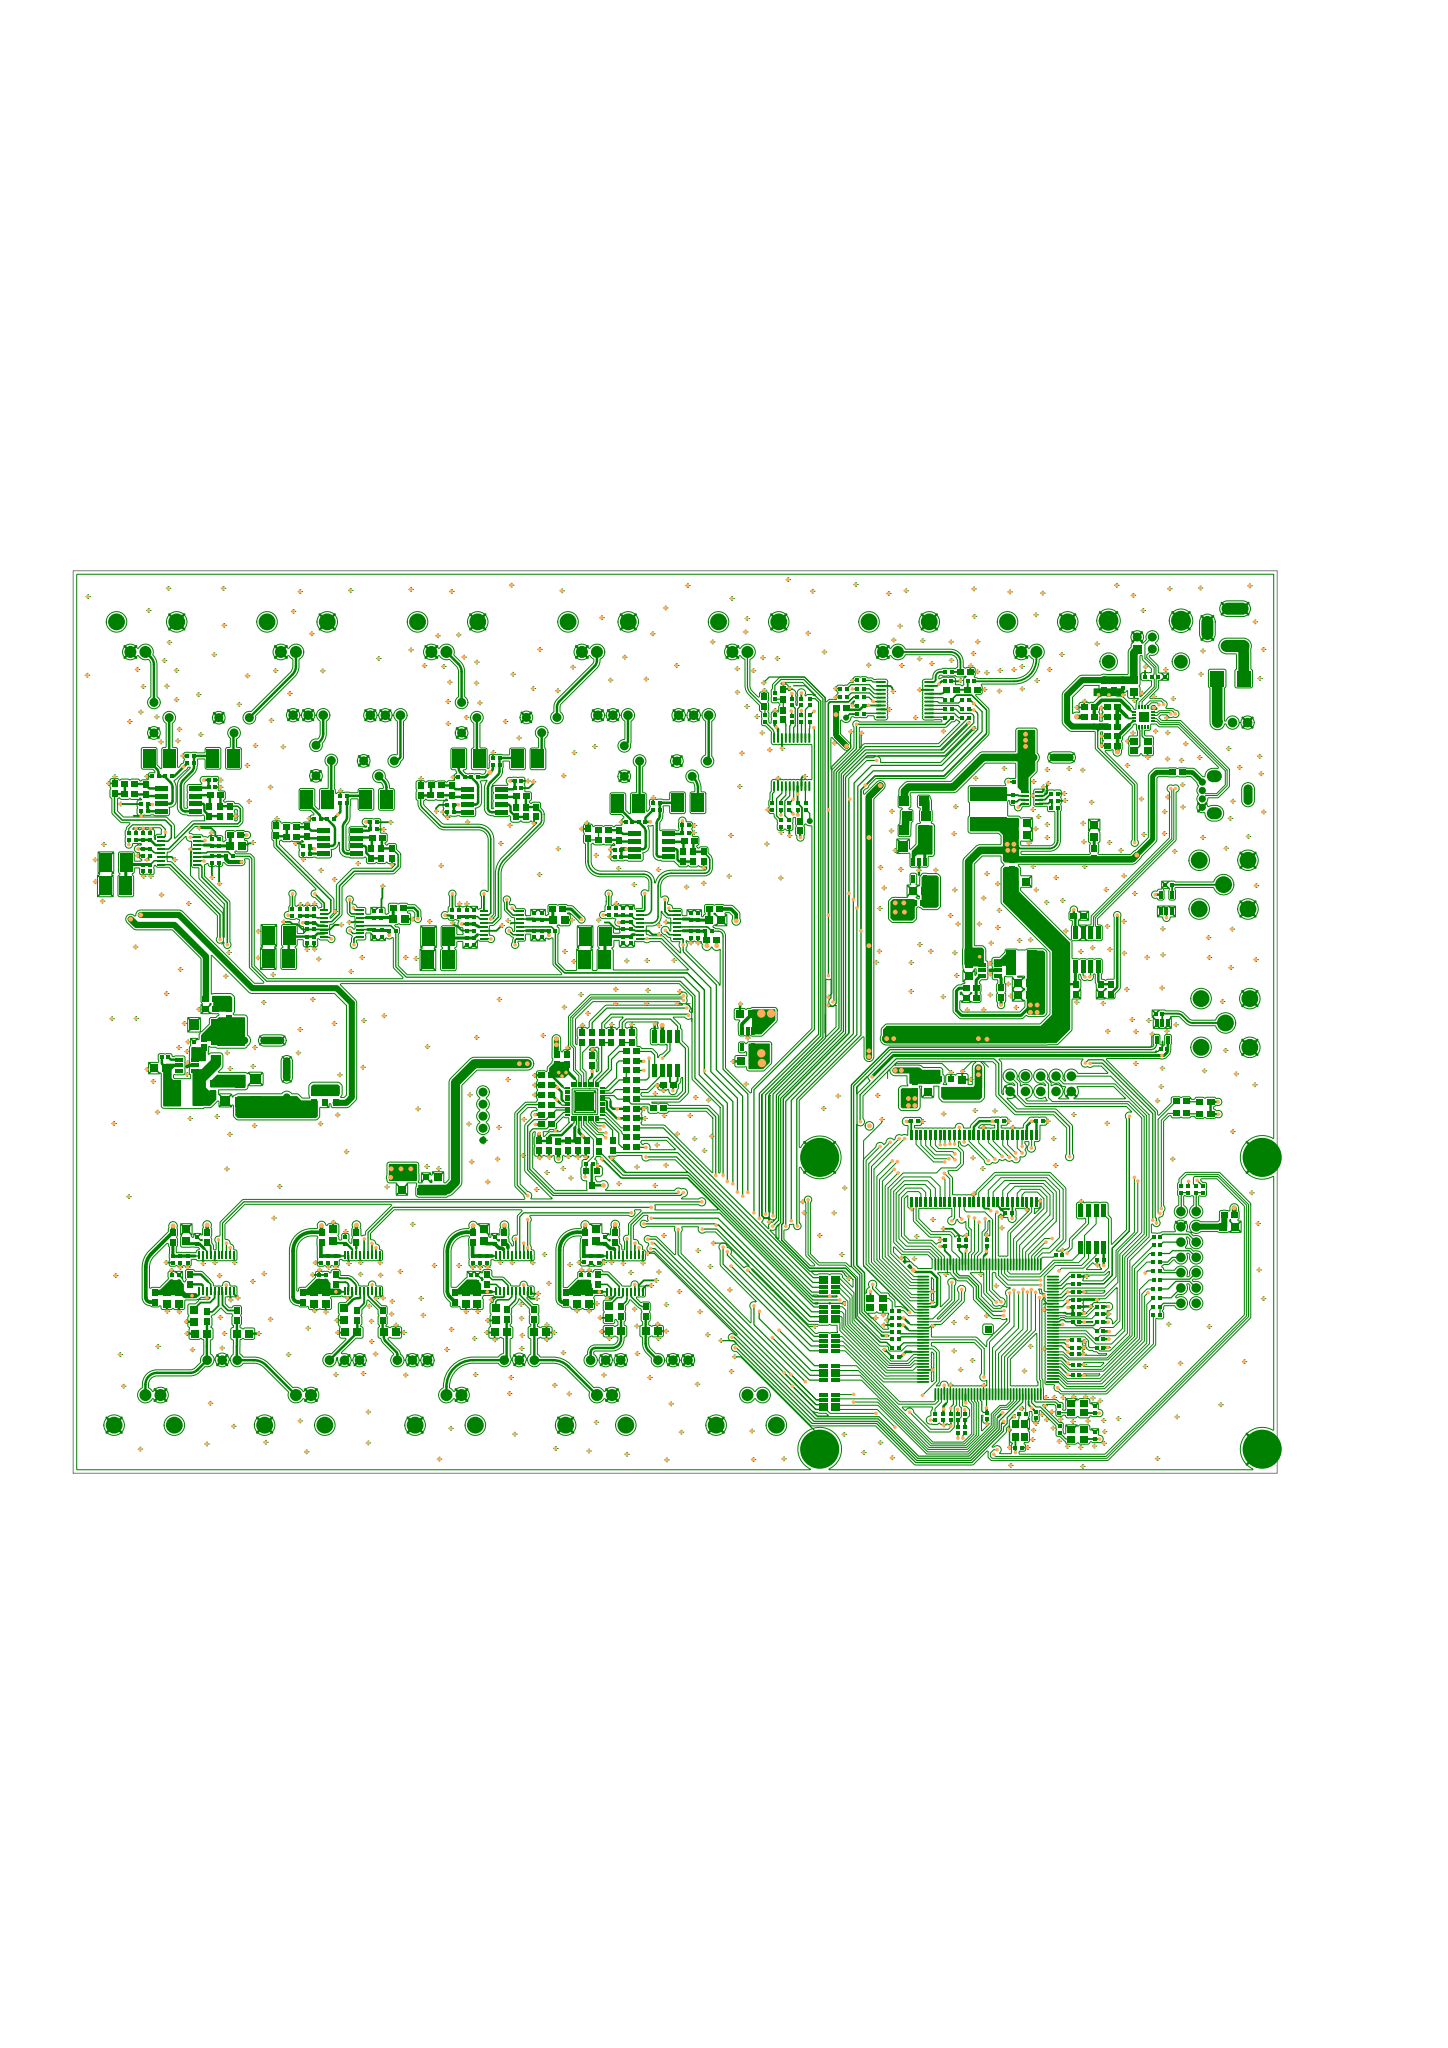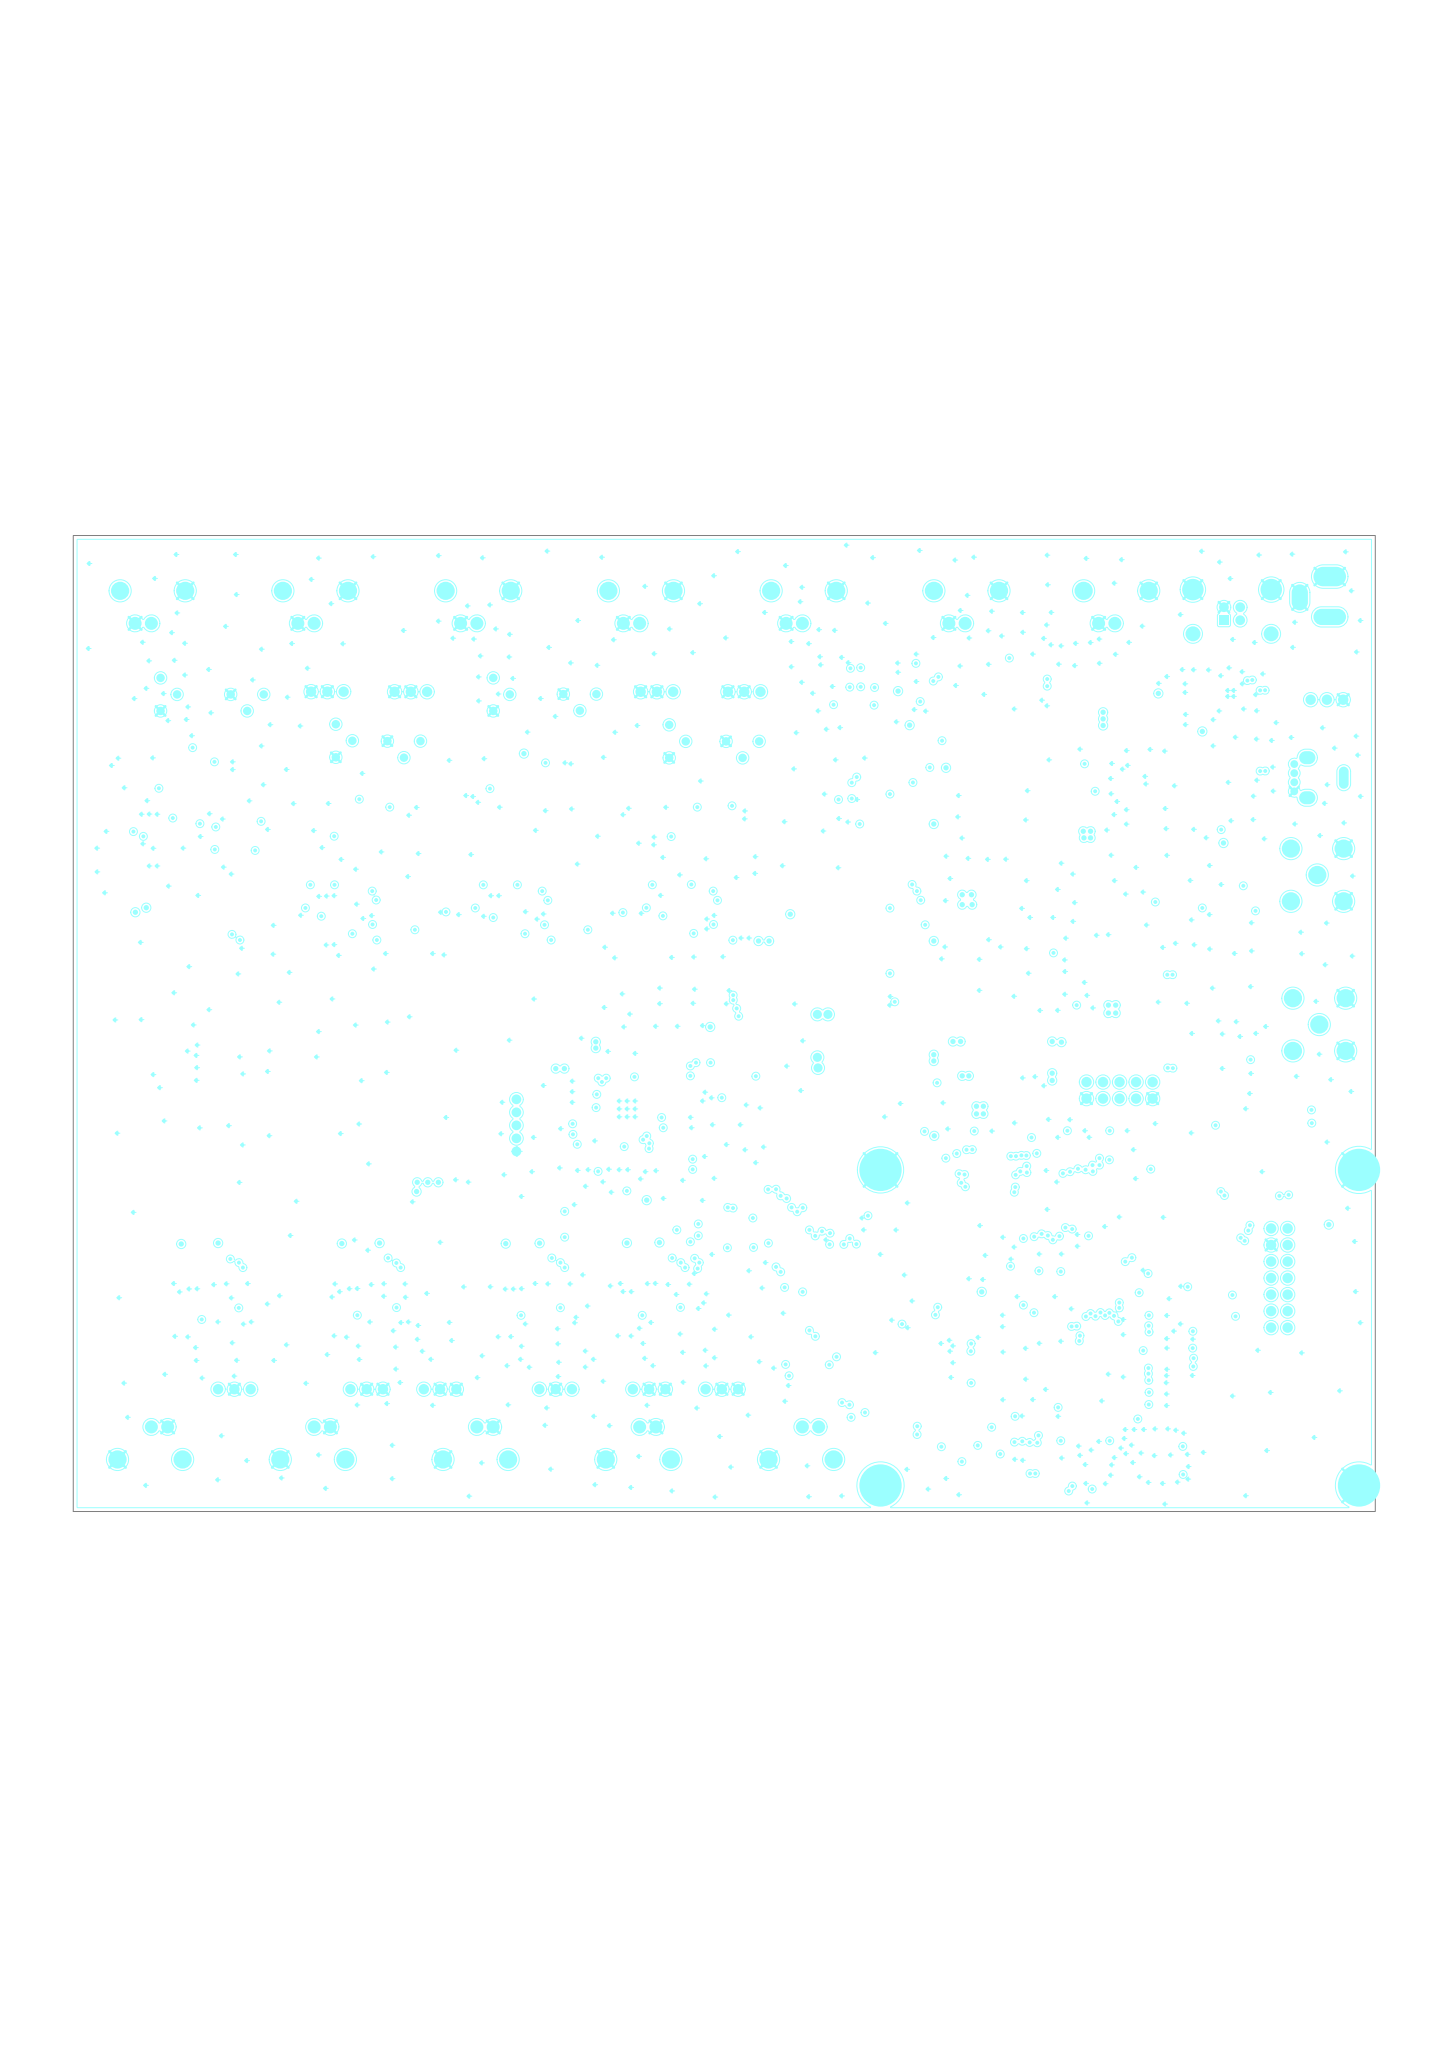Circuit board layout | Siemens PADS
Layer stack:
layer,name,type,plane,layer_thickness_mm,copper_thickness_mm,dielectric_constant
0,,,,0,,3.3
1,Top,ROUTING,NONE,0.254,0.0343,4.3
2,GND,ROUTING,NONE,0.254,0.0343,4.3
3,VCC,ROUTING,NONE,0.254,0.0343,4.3
4,Bottom,ROUTING,NONE,0,0.0343,3.3
Part placement:
Ref,PartType,Decal,X_mm,Y_mm,Rotation,Layer,Placed,Installed
C1,C0805,C0805,60.604,48.158,90,Top,True,True
C2,C0402,C0402,160.528,58.522,180,Top,True,True
C3,C0402,C0402,154.026,58.522,180,Top,True,True
C4,C0402,C0402,169.672,10.566,270,Top,True,True
C5,C0603,C0603,12.012,112.795,90,Top,True,True
C6,C0402,C0402,139.725,58.471,180,Top,True,True
C7,C0402,C0402,155.397,43.18,0,Top,True,True
C8,C0402,C0402,166.573,25.146,180,Top,True,True
C11,C0805,C0805,192.051,40.986,0,Top,True,True
C13,C0603,C0603,171.225,131.825,270,Top,True,True
C14,C0603,C0603,172.825,131.825,270,Top,True,True
C15,C0603,C0603,173.397,127.301,180,Top,True,True
C16,C0402,C0402,151.74,38.252,270,Top,True,True
C17,C0402,C0402,138.532,34.798,315,Top,True,True
C18,C0603,C0603,173.457,125.701,180,Top,True,True
C19,C0402,C0402,16.358,32.41,90,Top,True,True
C20,C0402,C0402,147.164,38.253,270,Top,True,True
C21,C0805,C0805,111.76,76.302,180,Top,True,True
C22,C0402,C0402,166.573,30.124,180,Top,True,True
C23,C0402,C0402,166.564,16.253,180,Top,True,True
C24,C0805,C0805,140.462,96.825,180,Top,True,True
C25,C0805,C0805,111.862,68.478,180,Top,True,True
C26,C0603,C0603,173.487,122.501,180,Top,True,True
C27,C0603,C0603,173.447,120.901,180,Top,True,True
C29,C0402,C0402,11.837,111.22,180,Top,True,True
C30,C0805,C0805,147.625,64.414,270,Top,True,True
C31,C0603,C0603,41.758,61.57,90,Top,True,True
C32,C1206,C1206,30.274,61.933,90,Top,True,True
C33,C0402,C0402,166.522,20.879,180,Top,True,True
C34,C0402,C0402,136.55,24.638,0,Top,True,True
C35,EC-SMD-D6.3,EC-SMD-D6.3,35.474,64.133,270,Top,True,True
C36,C0402,C0402,136.55,25.806,180,Top,True,True
C37,C0402,C0402,145.754,9.347,270,Top,True,True
C38,C0402,C0402,166.522,19.761,0,Top,True,True
C39,C0402,C0402,166.573,28.854,0,Top,True,True
C40,C0402,C0402,144.764,38.253,90,Top,True,True
C41,C0402,C0402,148.364,38.253,270,Top,True,True
C42,C0402,C0402,166.573,27.686,180,Top,True,True
C43,C0603,C0603,169.597,127.301,180,Top,True,True
C44,C0805,C0805,148.742,83.617,270,Top,True,True
C45,C0805,C0805,157.942,81.417,180,Top,True,True
C46,C0805,C0805,157.942,79.417,180,Top,True,True
C47,C0402,C0402,151.754,9.547,270,Top,True,True
C48,C0402,C0402,144.554,9.347,270,Top,True,True
C49,C0402,C0402,136.55,19.406,180,Top,True,True
C50,C0402,C0402,166.564,18.053,0,Top,True,True
C51,C0603,C0603,83.801,53.575,90,Top,True,True
C52,C0402,C0402,159.863,9.671,270,Top,True,True
C53,C0402,C0402,166.573,26.518,0,Top,True,True
C54,C0402,C0402,166.522,22.079,0,Top,True,True
C55,C0603,C0603,82.201,53.575,90,Top,True,True
C56,C0603,C0603,82.093,69.596,270,Top,True,True
C57,C0402,C0402,67.564,35.56,270,Top,True,True
C58,C0805,C0805,71,23.4,0,Top,True,True
C59,C0402,C0402,169.723,6.248,270,Top,True,True
C60,C0402,C0402,157.063,4.271,180,Top,True,True
C61,C0603,C0603,23.249,64.758,270,Top,True,True
C62,C0805,C0805,14.474,67.333,180,Top,True,True
C63,C0603,C0603,77.775,64.516,0,Top,True,True
C64,C0603,C0603,86.201,69.425,270,Top,True,True
C65,C0805,C0805,169.596,106.756,90,Top,True,True
C66,C0402,C0402,23.037,102.02,270,Top,True,True
C67,C0402,C0402,24.237,102.02,270,Top,True,True
C68,C0402,C0402,10.437,105.82,90,Top,True,True
C69,C0402,C0402,68.783,35.56,270,Top,True,True
C70,C0402,C0402,12.837,105.82,90,Top,True,True
C71,C0603,C0603,93.576,59,180,Top,True,True
C72,C0603,C0603,85.401,53.575,90,Top,True,True
C73,C0603,C0603,77.775,66.142,0,Top,True,True
C74,C0603,C0603,77.775,62.89,0,Top,True,True
C75,C0603,C0603,93.601,60.575,180,Top,True,True
C76,C0603,C0603,77.401,53.575,90,Top,True,True
C77,C0603,C0603,79.001,53.575,90,Top,True,True
C78,C0402,C0402,77.83,92.569,90,Top,True,True
C79,C0603,C0603,97.993,64.516,0,Top,True,True
C80,C0402,C0402,170.622,35.425,180,Top,True,True
C81,C0603,C0603,166.218,92.659,0,Top,True,True
C82,C0603,C0603,170.688,81.28,270,Top,True,True
C83,C0603,C0603,166.624,81.28,270,Top,True,True
C84,C0402,C0402,130.781,127.581,180,Top,True,True
C85,C0402,C0402,12.837,103.22,90,Top,True,True
C86,C0402,C0402,11.637,103.22,90,Top,True,True
C87,C0402,C0402,65.333,90.74,90,Top,True,True
C88,C0402,C0402,23.037,114.02,0,Top,True,True
C89,C0402,C0402,76.61,92.569,90,Top,True,True
C90,C0402,C0402,66.552,90.74,90,Top,True,True
C91,C0402,C0402,11.637,105.82,90,Top,True,True
C92,C0805,C0805,27.037,104.22,0,Top,True,True
C93,C0402,C0402,24.237,104.82,90,Top,True,True
C94,C0805,C0805,80.622,91.935,0,Top,True,True
C95,C0402,C0402,23.037,104.82,90,Top,True,True
C96,C0402,C0402,145.339,131.623,0,Top,True,True
C97,C1206,C1206,141.462,104.225,180,Top,True,True
C98,C0402,C0402,66.533,88.404,90,Top,True,True
C99,C0603,C0603,6.862,114.645,270,Top,True,True
C100,TAN_C3528,TAN_C3528,60.622,85.335,180,Top,True,True
C101,C0402,C0402,11.637,100.62,90,Top,True,True
C102,TAN_C3528,TAN_C3528,7.037,97.62,180,Top,True,True
C103,C0402,C0402,12.837,100.62,90,Top,True,True
C104,C0402,C0402,120.351,110.801,270,Top,True,True
C105,TAN_C3528,TAN_C3528,7.137,101.47,180,Top,True,True
C106,C0402,C0402,65.333,88.404,90,Top,True,True
C107,C0402,C0402,77.83,89.623,270,Top,True,True
C108,TAN_C3528,TAN_C3528,60.722,89.185,180,Top,True,True
C109,C0402,C0402,76.61,89.623,270,Top,True,True
C110,C0603,C0603,22.637,109.22,90,Top,True,True
C111,C0805,C0805,18.796,39.522,270,Top,True,True
C112,C0805,C0805,17.577,29.159,270,Top,True,True
C113,C0402,C0402,66.345,35.56,270,Top,True,True
C114,C0402,C0402,67.158,32.41,90,Top,True,True
C115,C0805,C0805,67.158,29.159,270,Top,True,True
C116,C0402,C0402,66.04,32.41,90,Top,True,True
C117,C0402,C0402,20.625,38.71,270,Top,True,True
C118,C0402,C0402,17.577,32.41,90,Top,True,True
C119,C0805,C0805,20,26.2,90,Top,True,True
C120,C0805,C0805,15.545,29.159,270,Top,True,True
C121,C0402,C0402,70.002,38.71,270,Top,True,True
C122,C0805,C0805,65.227,29.159,270,Top,True,True
C123,C0805,C0805,21.2,23.2,0,Top,True,True
C124,C0805,C0805,68.174,39.522,270,Top,True,True
C125,C0603,C0603,19.4,31.4,90,Top,True,True
C126,C0402,C0402,11.837,110.02,180,Top,True,True
C127,TAN_C3528,TAN_C3528,24.919,118.824,0,Top,True,True
C128,C0402,C0402,64.114,93.077,90,Top,True,True
C129,C0402,C0402,65.333,93.077,90,Top,True,True
C130,C0402,C0402,66.552,93.077,90,Top,True,True
C131,C0805,C0805,28.2,23.2,0,Top,True,True
C132,C0805,C0805,70.2,26.4,90,Top,True,True
C133,C0402,C0402,51.208,92.911,90,Top,True,True
C134,TAN_C3528,TAN_C3528,14.319,118.824,0,Top,True,True
C135,C0603,C0603,26.037,109.22,90,Top,True,True
C136,C0402,C0402,40.032,90.93,90,Top,True,True
C137,C0805,C0805,77.6,23.4,0,Top,True,True
C138,C0603,C0603,68.783,31.394,90,Top,True,True
C139,C0402,C0402,43.586,35.56,270,Top,True,True
C140,C0402,C0402,17.78,35.56,270,Top,True,True
C141,C0402,C0402,18.999,35.56,270,Top,True,True
C142,C0402,C0402,16.561,35.56,270,Top,True,True
C143,C0805,C0805,46.2,23.4,0,Top,True,True
C144,C0402,C0402,41.148,35.56,270,Top,True,True
C145,C0402,C0402,42.367,35.56,270,Top,True,True
C146,C0402,C0402,41.961,32.41,90,Top,True,True
C147,C0805,C0805,41.961,29.159,270,Top,True,True
C148,C0402,C0402,50.04,92.911,90,Top,True,True
C150,C0402,C0402,40.843,32.41,90,Top,True,True
C151,C0402,C0402,45.212,38.71,270,Top,True,True
C153,C0805,C0805,40.03,29.159,270,Top,True,True
C154,C0805,C0805,43.18,39.522,270,Top,True,True
C155,C0805,C0805,157.378,106.001,0,Top,True,True
C156,C0805,C0805,45,26.4,90,Top,True,True
C157,C0402,C0402,114.951,125.401,270,Top,True,True
C158,C0805,C0805,52.6,23.4,0,Top,True,True
C159,C0603,C0603,43.586,31.394,90,Top,True,True
C160,C0402,C0402,87.274,35.56,270,Top,True,True
C161,C0805,C0805,90,23.6,0,Top,True,True
C162,C0402,C0402,84.818,35.605,270,Top,True,True
C163,C0402,C0402,86.055,35.56,270,Top,True,True
C164,C0402,C0402,85.649,32.41,90,Top,True,True
C165,EC-SMD-D6.3,EC-SMD-D6.3,161.178,118.965,0,Top,True,True
C166,EC-SMD-D6.3,EC-SMD-D6.3,30.074,71.933,0,Top,True,True
C167,C0805,C0805,85.649,29.159,270,Top,True,True
C168,C0402,C0402,84.418,32.405,90,Top,True,True
C169,C1206,C1206,23.674,74.533,180,Top,True,True
C170,C0402,C0402,88.392,38.71,270,Top,True,True
C171,C0805,C0805,83.618,29.205,270,Top,True,True
C172,C0603,C0603,22.024,77.133,0,Top,True,True
C173,C0805,C0805,86.868,39.522,270,Top,True,True
C174,C0805,C0805,89.002,26.822,90,Top,True,True
C175,C0805,C0805,96.088,23.622,0,Top,True,True
C176,C0603,C0603,87.173,31.394,90,Top,True,True
C177,C0402,C0402,116.551,125.401,90,Top,True,True
C179,C0402,C0402,145.381,133.181,180,Top,True,True
C180,C0402,C0402,149.139,131.623,0,Top,True,True
C183,C0402,C0402,116.551,129.201,90,Top,True,True
C184,C0402,C0402,38.864,90.93,90,Top,True,True
C190,C0805,C0805,141.935,64.414,270,Top,True,True
C192,C0805,C0805,54.104,92.138,0,Top,True,True
C194,C0805,C0805,157.277,98.349,0,Top,True,True
C196,C0805,C0805,157.378,108.001,0,Top,True,True
C204,C0805,C0805,54.604,48.159,270,Top,True,True
C228,C0402,C0402,156.178,112.165,270,Top,True,True
C229,C0402,C0402,40.013,88.644,90,Top,True,True
C230,TAN_C3528,TAN_C3528,34.104,85.538,180,Top,True,True
C231,C0402,C0402,38.813,88.644,90,Top,True,True
C232,C0402,C0402,51.259,89.66,270,Top,True,True
C233,TAN_C3528,TAN_C3528,34.204,89.388,180,Top,True,True
C234,C0402,C0402,50.04,89.66,270,Top,True,True
C235,C0402,C0402,37.695,93.216,90,Top,True,True
C236,C0402,C0402,38.864,93.216,90,Top,True,True
C237,C0402,C0402,40.032,93.216,90,Top,True,True
C238,C0402,C0402,102.555,92.513,90,Top,True,True
C240,C0402,C0402,91.379,90.989,90,Top,True,True
C241,C0402,C0402,103.774,92.513,90,Top,True,True
C242,C0402,C0402,92.598,90.989,90,Top,True,True
C243,C0805,C0805,106.631,91.935,0,Top,True,True
C244,C0402,C0402,92.579,88.652,90,Top,True,True
C245,TAN_C3528,TAN_C3528,86.631,85.335,180,Top,True,True
C246,C0402,C0402,91.379,88.652,90,Top,True,True
C247,C0402,C0402,102.555,89.566,270,Top,True,True
C248,TAN_C3528,TAN_C3528,86.731,89.185,180,Top,True,True
C249,C0402,C0402,103.774,89.566,270,Top,True,True
C250,C0402,C0402,90.16,93.326,90,Top,True,True
C251,C0402,C0402,91.398,93.326,90,Top,True,True
C252,C0402,C0402,92.598,93.326,90,Top,True,True
C253,C0402,C0402,23.037,115.22,0,Top,True,True
C254,C0603,C0603,62.859,112.653,90,Top,True,True
C255,C0402,C0402,62.684,111.078,180,Top,True,True
C256,TAN_C3528,TAN_C3528,65.749,118.735,0,Top,True,True
C257,C0603,C0603,57.709,114.3,270,Top,True,True
C258,C0402,C0402,73.884,113.878,0,Top,True,True
C259,C0603,C0603,73.484,109.078,90,Top,True,True
C260,C0402,C0402,62.684,109.878,180,Top,True,True
C261,TAN_C3528,TAN_C3528,75.503,118.735,0,Top,True,True
C262,C0603,C0603,76.884,109.078,90,Top,True,True
C263,C0402,C0402,73.884,115.078,0,Top,True,True
C264,C0603,C0603,38.908,105.771,90,Top,True,True
C265,C0402,C0402,38.733,104.196,180,Top,True,True
C266,TAN_C3528,TAN_C3528,40.533,111.996,0,Top,True,True
C267,C0603,C0603,33.758,107.621,270,Top,True,True
C268,C0402,C0402,49.933,106.996,0,Top,True,True
C269,C0603,C0603,49.533,102.196,90,Top,True,True
C270,C0402,C0402,38.733,102.996,180,Top,True,True
C271,TAN_C3528,TAN_C3528,50.333,111.996,0,Top,True,True
C272,C0603,C0603,52.933,102.196,90,Top,True,True
C273,C0402,C0402,49.933,108.196,0,Top,True,True
C274,C0603,C0603,90.679,105.238,90,Top,True,True
C275,C0402,C0402,90.504,103.663,180,Top,True,True
C276,TAN_C3528,TAN_C3528,92.179,111.288,0,Top,True,True
C277,C0603,C0603,85.529,107.088,270,Top,True,True
C278,C0402,C0402,101.704,106.463,0,Top,True,True
C279,C0603,C0603,101.304,101.663,90,Top,True,True
C280,C0402,C0402,90.504,102.463,180,Top,True,True
C281,TAN_C3528,TAN_C3528,102.079,111.438,0,Top,True,True
C282,C0603,C0603,104.704,101.663,90,Top,True,True
C283,C0402,C0402,101.704,107.663,0,Top,True,True
C350,C0402,C0402,181.17,70.591,180,Top,True,True
COXL_IN1,BNC-Q9-V,BNC-Q9-V,112,136.5,180,Top,False,True
COXL_IN2,BNC-Q9-V,BNC-Q9-V,137,136.5,180,Top,False,True
COXL_OUT1,BNC-Q9-V,BNC-Q9-V,112,13,0,Top,False,True
COXL_OUT2,BNC-Q9-V,BNC-Q9-V,160,136.5,180,Top,False,True
ESD7,L0402,L0402,174.346,131.013,270,Top,True,True
ESD8,L0402,L0402,180.8,132.4,0,Top,True,True
ESD9,L0402,L0402,178.6,132.4,180,Top,True,True
ESD14,L0402,L0402,180.37,76.391,180,Top,True,True
ESD15,L0402,L0402,181.955,97.81,180,Top,True,True
H1,HOLE3.5,HOLE3.5,124,4,0,Top,True,True
H2,HOLE3.5,HOLE3.5,197.5,52.5,0,Top,False,True
H3,HOLE3.5,HOLE3.5,124,52.5,0,Top,True,True
H4,HOLE3.5,HOLE3.5,197.5,4,0,Top,False,True
IN1,BNC-Q9-V,BNC-Q9-V,12,136.5,180,Top,False,True
IN2,BNC-Q9-V,BNC-Q9-V,37,136.5,180,Top,False,True
IN3,BNC-Q9-V,BNC-Q9-V,62,136.5,180,Top,False,True
IN4,BNC-Q9-V,BNC-Q9-V,87,136.5,180,Top,False,True
IN5,CN25-3VS,CN25-3VS,41.533,125.996,180,Top,True,True
IN6,CN25-3VS,CN25-3VS,54.356,125.984,180,Top,True,True
IN7,CN25-3VS,CN25-3VS,92.151,125.984,180,Top,True,True
IN8,CN25-3VS,CN25-3VS,105.562,125.984,180,Top,True,True
J1,CN254-14AVD,CN254-14AVD,184,43.5,90,Top,True,True
J2,USB-A-VS,USB-A-VS,187.554,112.776,90,Top,False,True
J5,CN25-3VS,CN25-3VS,22.25,18.796,0,Top,True,True
J6,CN25-3VS,CN25-3VS,71.6,18.8,0,Top,True,True
J11,BNC-V-5,BNC-V-5,191.4,74.84,90,Top,False,True
J12,BNC-V-5,BNC-V-5,191.09,97.83,90,Top,False,True
JTAG1,CN254-10AVD,CN254-10AVD,165.8,66,0,Top,True,True
JTAG2,PH20-05P,PH20-05P,68.072,55.348,90,Top,True,True
L2,L0603,L0603,171.807,124.101,0,Top,True,True
L3,L0603,L0603,155.956,100.381,90,Top,True,True
L4,L0603,L0603,40.03,61.57,90,Top,True,True
L5,L0603,L0603,139.802,65.126,270,Top,True,True
L6,NR4030,NR4030,157.542,84.817,0,Top,True,True
L7,L0603,L0603,80.293,67.946,90,Top,True,True
L8,L0603,L0603,141.211,94.759,180,Top,True,True
L9,L0603,L0603,66.446,38.405,90,Top,True,True
L10,L0603,L0603,184.252,116.484,180,Top,True,True
L11,INDUCTOR_5X5_SMD,INDUCTOR_5X5_SMD,18.874,63.133,0,Top,True,True
L12,L0603,L0603,106.883,88.697,180,Top,True,True
L13,L0603,L0603,25.874,75.533,90,Top,True,True
L14,L0603,L0603,120.751,108.401,270,Top,True,True
L15,L0603,L0603,169.596,103.861,270,Top,True,True
L16,L0603,L0603,43.586,61.57,90,Top,True,True
L18,L0603,L0603,22.047,78.842,0,Top,True,True
L20,L0603,L0603,16.561,38.405,90,Top,True,True
L21,L0603,L0603,191.211,42.926,0,Top,True,True
L22,L0603,L0603,13.614,28.448,90,Top,True,True
L23,NR6045T,NR6045T,151.978,110.365,270,Top,True,True
L24,L0603,L0603,63.398,28.448,90,Top,True,True
L25,L0603,L0603,41.25,38.405,90,Top,True,True
L26,L0603,L0603,38.202,28.448,90,Top,True,True
L27,L0603,L0603,85.039,38.405,90,Top,True,True
L28,L0603,L0603,81.818,28.405,90,Top,True,True
L29,L0603,L0603,128.381,127.181,180,Top,True,True
LED1,LED_603,LED_603,188.925,59.741,180,Top,True,True
LED2,LED_603,LED_603,188.925,61.741,180,Top,True,True
OUT1,BNC-Q9-V,BNC-Q9-V,12,13,0,Top,False,True
OUT2,BNC-Q9-V,BNC-Q9-V,37,13,0,Top,False,True
OUT3,BNC-Q9-V,BNC-Q9-V,62,13,0,Top,False,True
OUT4,BNC-Q9-V,BNC-Q9-V,87,13,0,Top,False,True
OUT5,CN25-3VS,CN25-3VS,42.57,18.796,0,Top,True,True
OUT6,CN25-3VS,CN25-3VS,53.848,18.796,0,Top,True,True
OUT7,CN25-3VS,CN25-3VS,85.954,18.796,0,Top,True,True
OUT8,CN25-3VS,CN25-3VS,97.13,18.796,0,Top,True,True
P1,CN25-3VS,CN25-3VS,195.072,124.765,180,Top,True,True
P2,USB2-D,USB2-D,178,141.69,180,Top,False,True
P4,DC005,DC005,193,143.69,0,Top,False,True
R1,R0402,R0402,170.586,25.095,0,Top,True,True
R5,R0402,R0402,163.83,10.617,90,Top,True,True
R6,R0402,R0402,136.601,27.026,0,Top,True,True
R7,R0402,R0402,179.984,26.264,180,Top,True,True
R8,R0402,R0402,180.025,39.329,180,Top,True,True
R9,R0603,R0603,21.674,72.333,270,Top,True,True
R10,R0603,R0603,167.997,125.701,0,Top,True,True
R11,R0402,R0402,180.025,37.929,180,Top,True,True
R12,R0603,R0603,154.142,79.017,90,Top,True,True
R13,R0603,R0603,149.992,80.617,180,Top,True,True
R14,R0603,R0603,149.992,79.017,180,Top,True,True
R15,R0402,R0402,179.984,36.525,180,Top,True,True
R16,R0402,R0402,157.663,9.871,0,Top,True,True
R17,R0402,R0402,163.855,7.29,90,Top,True,True
R18,R0402,R0402,179.984,35.103,180,Top,True,True
R19,R0402,R0402,136.564,23.453,0,Top,True,True
R20,R0402,R0402,180.025,32.129,180,Top,True,True
R21,R0402,R0402,179.984,30.632,180,Top,True,True
R22,R0402,R0402,179.984,33.63,180,Top,True,True
R23,R0402,R0402,85.751,51.47,0,Top,True,True
R24,R0402,R0402,170.536,20.879,180,Top,True,True
R25,R0402,R0402,170.586,22.301,0,Top,True,True
R26,R0402,R0402,170.586,23.571,0,Top,True,True
R27,R0402,R0402,166.573,31.496,0,Top,True,True
R28,R0402,R0402,170.536,27.698,0,Top,True,True
R29,R0402,R0402,170.536,26.498,0,Top,True,True
R30,R0402,R0402,166.573,32.715,0,Top,True,True
R31,R0402,R0402,179.984,29.159,180,Top,True,True
R32,R0402,R0402,179.984,27.686,180,Top,True,True
R33,R0402,R0402,136.564,20.853,180,Top,True,True
R34,R0402,R0402,146.954,9.347,90,Top,True,True
R35,R0402,R0402,148.154,9.347,90,Top,True,True
R36,R0402,R0402,148.133,7.163,270,Top,True,True
R37,R0402,R0402,146.964,7.163,270,Top,True,True
R38,R0603,R0603,93.551,65.375,180,Top,True,True
R39,R0402,R0402,163.728,36.271,0,Top,True,True
R40,R0402,R0402,185.255,47.193,90,Top,True,True
R41,R0603,R0603,184.85,59.816,180,Top,True,True
R42,R0603,R0603,184.85,61.816,180,Top,True,True
R43,R0402,R0402,187.655,47.193,90,Top,True,True
R44,R0603,R0603,93.551,62.175,180,Top,True,True
R45,R0603,R0603,27.2,25.4,90,Top,True,True
R46,R0603,R0603,80.601,55.175,270,Top,True,True
R47,R0603,R0603,93.551,63.775,180,Top,True,True
R48,R0603,R0603,93.523,70.104,180,Top,True,True
R49,R0603,R0603,77.775,61.265,0,Top,True,True
R50,R0603,R0603,93.601,54.175,180,Top,True,True
R51,R0603,R0603,89.601,53.575,90,Top,True,True
R52,R0603,R0603,93.539,55.812,180,Top,True,True
R53,R0603,R0603,10.237,112.82,180,Top,True,True
R54,R0603,R0603,22.225,25.175,90,Top,True,True
R55,R0603,R0603,93.576,57.4,180,Top,True,True
R56,R0603,R0603,24.437,109.22,90,Top,True,True
R58,R0603,R0603,91.201,73.225,270,Top,True,True
R59,R0603,R0603,87.801,73.175,270,Top,True,True
R61,R0603,R0603,86.201,73.225,270,Top,True,True
R62,R0603,R0603,84.531,73.254,270,Top,True,True
R63,R0603,R0603,79.401,57.975,180,Top,True,True
R64,R0603,R0603,72,25.6,90,Top,True,True
R65,R0603,R0603,76.6,25.6,90,Top,True,True
R66,R0603,R0603,79.4,59.588,180,Top,True,True
R67,R0603,R0603,91.897,68.529,0,Top,True,True
R68,R0603,R0603,92.801,71.575,90,Top,True,True
R69,R0603,R0603,89.401,71.575,90,Top,True,True
R70,R0402,R0402,143.154,9.347,90,Top,True,True
R71,R0402,R0402,136.564,22.253,0,Top,True,True
R72,R0603,R0603,93.523,66.954,180,Top,True,True
R73,R0603,R0603,8.587,114.62,0,Top,True,True
R74,R0603,R0603,97.993,60.655,180,Top,True,True
R75,R0603,R0603,87.401,55.175,270,Top,True,True
R76,R0603,R0603,172.314,79.654,90,Top,True,True
R77,R0402,R0402,117.551,110.801,90,Top,True,True
R78,R0402,R0402,117.551,108.001,90,Top,True,True
R79,R0402,R0402,116.151,110.801,90,Top,True,True
R80,R0402,R0402,118.951,108.001,90,Top,True,True
R81,R0402,R0402,118.951,110.801,90,Top,True,True
R82,R0402,R0402,122.351,128.201,270,Top,True,True
R83,R0402,R0402,120.951,125.401,270,Top,True,True
R84,R0402,R0402,120.951,128.201,270,Top,True,True
R85,R0402,R0402,119.38,128.168,270,Top,True,True
R86,R0402,R0402,119.38,125.368,270,Top,True,True
R87,R0402,R0402,121.751,110.801,90,Top,True,True
R88,R0603,R0603,117.951,125.201,90,Top,True,True
R89,R0603,R0603,114.751,127.401,90,Top,True,True
R90,R0603,R0603,117.951,128.601,90,Top,True,True
R91,R0402,R0402,25.933,102.54,0,Top,True,True
R92,R0402,R0402,9.237,105.82,270,Top,True,True
R93,R0603,R0603,27.737,106.07,180,Top,True,True
R94,R0603,R0603,81.322,93.785,180,Top,True,True
R95,R0402,R0402,62.894,93.077,270,Top,True,True
R96,R0402,R0402,79.553,90.17,0,Top,True,True
R97,R0603,R0603,54.804,93.988,180,Top,True,True
R98,R0402,R0402,15.837,115.82,180,Top,True,True
R99,R0402,R0402,13.637,115.82,180,Top,True,True
R100,R0402,R0402,19.519,118.024,0,Top,True,True
R101,R0402,R0402,36.425,93.216,270,Top,True,True
R102,R0402,R0402,53.035,90.195,0,Top,True,True
R103,R0603,R0603,107.331,93.785,180,Top,True,True
R104,R0402,R0402,88.941,93.326,270,Top,True,True
R105,R0402,R0402,105.537,90.094,0,Top,True,True
R106,R0603,R0603,24.462,112.645,180,Top,True,True
R107,R0402,R0402,19.519,119.224,180,Top,True,True
R108,R0603,R0603,22.25,38.405,90,Top,True,True
R109,R0603,R0603,61.084,112.678,180,Top,True,True
R110,R0402,R0402,66.684,115.678,180,Top,True,True
R111,R0603,R0603,59.45,114.315,0,Top,True,True
R112,R0402,R0402,64.484,115.678,180,Top,True,True
R113,R0603,R0603,75.198,109.083,90,Top,True,True
R114,R0402,R0402,70.265,117.678,0,Top,True,True
R115,R0603,R0603,75.309,112.503,180,Top,True,True
R116,R0402,R0402,70.265,118.878,180,Top,True,True
R117,R0402,R0402,15.273,69.133,0,Top,True,True
R118,R0402,R0402,20.074,71.133,90,Top,True,True
R119,R0603,R0603,37.133,105.796,180,Top,True,True
R120,R0402,R0402,42.733,108.796,180,Top,True,True
R121,R0603,R0603,35.458,107.391,0,Top,True,True
R122,R0402,R0402,40.533,108.796,180,Top,True,True
R123,R0603,R0603,51.206,102.21,90,Top,True,True
R124,R0402,R0402,44.933,111.396,0,Top,True,True
R125,R0603,R0603,51.358,105.621,180,Top,True,True
R126,R0402,R0402,44.933,112.596,180,Top,True,True
R127,R0603,R0603,88.904,105.263,180,Top,True,True
R128,R0402,R0402,94.504,108.263,180,Top,True,True
R129,R0603,R0603,87.274,106.883,0,Top,True,True
R130,R0402,R0402,92.304,108.263,180,Top,True,True
R131,R0603,R0603,103.022,101.651,90,Top,True,True
R132,R0603,R0603,71.628,38.405,90,Top,True,True
R133,R0402,R0402,96.879,110.238,0,Top,True,True
R134,R0603,R0603,47.2,25.4,90,Top,True,True
R135,R0603,R0603,51.4,25.4,90,Top,True,True
R136,R0603,R0603,103.129,105.088,180,Top,True,True
R137,R0603,R0603,47.041,38.405,90,Top,True,True
R138,R0402,R0402,96.879,111.438,180,Top,True,True
R139,R0603,R0603,91.002,26.022,90,Top,True,True
R140,R0603,R0603,95.098,26.01,90,Top,True,True
R141,R0603,R0603,90.018,38.405,90,Top,True,True
R142,R0402,R0402,130.781,130.381,0,Top,True,True
R143,R0402,R0402,127.981,130.381,0,Top,True,True
R144,R0402,R0402,130.781,131.781,0,Top,True,True
R145,R0402,R0402,127.981,128.981,0,Top,True,True
R146,R0402,R0402,130.781,128.981,0,Top,True,True
R147,R0402,R0402,148.181,125.581,180,Top,True,True
R148,R0402,R0402,145.381,126.981,180,Top,True,True
R149,R0402,R0402,148.181,126.981,180,Top,True,True
R150,R0402,R0402,148.19,128.575,180,Top,True,True
R151,R0402,R0402,145.39,128.575,180,Top,True,True
R152,R0402,R0402,130.781,126.181,0,Top,True,True
R153,R0603,R0603,145.139,130.223,0,Top,True,True
R154,R0603,R0603,147.381,133.181,0,Top,True,True
R155,R0603,R0603,148.539,130.223,0,Top,True,True
R156,R0402,R0402,122.351,125.401,90,Top,True,True
R157,R0402,R0402,145.381,125.581,0,Top,True,True
R158,R0402,R0402,184.055,47.193,90,Top,True,True
R159,R0402,R0402,186.455,47.193,90,Top,True,True
R304,R0402,R0402,156.769,114.859,180,Top,True,True
R305,R0402,R0402,162.978,110.565,180,Top,True,True
R307,R0402,R0402,162.978,111.765,0,Top,True,True
R308,R0402,R0402,162.978,112.965,0,Top,True,True
RP1,RES/8/742,RES/8/742,124.765,22.758,270,Top,True,True
RP2,RES/8/742,RES/8/742,124.765,27.635,270,Top,True,True
RP3,RES/8/742,RES/8/742,124.765,32.512,270,Top,True,True
RP4,RES/8/742,RES/8/742,124.765,17.882,270,Top,True,True
RP5,RES/8/742,RES/8/742,124.765,13.005,270,Top,True,True
RV1,RV3225,RV3225,13.411,128.118,270,Top,True,True
RV2,RV3225,RV3225,29.261,125.578,180,Top,True,True
RV3,RV3225,RV3225,64.516,128.118,270,Top,True,True
RV4,RV3225,RV3225,80.358,125.625,180,Top,True,True
RV5,RV3225,RV3225,40.333,120.996,270,Top,True,True
RV6,RV3225,RV3225,53.333,118.396,180,Top,True,True
RV7,RV3225,RV3225,91.542,120.904,270,Top,True,True
RV8,RV3225,RV3225,105.359,118.364,180,Top,True,True
TP1,TP1,TP1,122.351,108.401,90,Top,True,True
TP2,TP1,TP1,128.381,125.581,0,Top,True,True
U1,TSOP54-II,TSOP54-II,149.61,50.703,270,Top,True,True
U3,QFN16-3X3,QFN16-3X3,177.797,125.701,90,Top,True,True
U4,SOT-23,SOT-23,87.071,50.19,180,Top,True,True
U5,SOP-8W,SOP-8W,171.188,43.669,270,Top,True,True
U6,SOT23-6,SOT23-6,152.302,83.597,90,Top,True,True
U7,CRY-3225,CRY-3225,132.436,27.534,0,Top,True,True
U8,SOT23-6,SOT23-6,18.934,67.793,90,Top,True,True
U9,CRY-3225,CRY-3225,167.919,11.557,180,Top,True,True
U10,TSOT23-8,TSOT23-8,159.294,112.281,180,Top,True,True
U11,SOT23B,SOT23B,145.766,65.481,180,Top,True,True
U12,QFN48-XU208,QFN48-XU208,85.001,61.775,90,Top,True,True
U13,SOP-8,SOP-8,170.282,89.814,270,Top,True,True
U14,SOP-8,SOP-8,100.401,72.575,270,Top,True,True
U15,SOT23-5,SOT23-5,112.983,73.582,180,Top,True,True
U16,WM8804G,WM8804G,119.351,118.201,90,Top,True,True
U17,TSSOP16,TSSOP16,17.637,103.42,180,Top,True,True
U18,TSSOP16,TSSOP16,71.222,91.135,180,Top,True,True
U19,SOP-8,SOP-8,14.637,113.82,0,Top,True,True
U20,TSSOP16,TSSOP16,44.704,91.338,180,Top,True,True
U21,TSSOP16,TSSOP16,97.231,91.135,180,Top,True,True
U22,CRY-3225,CRY-3225,157.988,6.096,90,Top,True,True
U23,CRY-3225,CRY-3225,167.919,7.196,180,Top,True,True
U24,SOP-8,SOP-8,65.484,113.678,0,Top,True,True
U25,SOP-8,SOP-8,41.533,106.796,0,Top,True,True
U26,SOP-8,SOP-8,93.304,106.263,0,Top,True,True
U27,TSSOP-20,TSSOP-20,23.774,33.223,90,Top,True,True
U28,TSSOP-20,TSSOP-20,73.152,33.223,90,Top,True,True
U30,TSSOP-20,TSSOP-20,47.955,33.223,90,Top,True,True
U31,TSSOP-20,TSSOP-20,91.618,33.205,90,Top,True,True
U32,SOT23B,SOT23B,58.594,49.189,180,Top,True,True
U33,WM8804G,WM8804G,138.181,128.581,0,Top,True,True
U34,SOT23-5,SOT23-5,141.462,101.625,180,Top,True,True
U35,SOT23-5,SOT23-5,181.86,74.841,180,Top,True,True
U36,SOT23-5,SOT23-5,180.645,93.37,0,Top,True,True
U47,PGL12G-LQFP144,PGL12G-LQFP144,162.744,15.183,180,Top,True,True
Y1,CRY_3225,CRY_3225,177.382,120.889,180,Top,True,True
ZD1,SOD123,SOD123,27.674,63.333,90,Top,True,True
ZD2,SOD123,SOD123,139.687,111.65,0,Top,True,True
ZD3,SOD123,SOD123,25.274,63.533,270,Top,True,True
ZD4,SOD123,SOD123,23.674,70.333,90,Top,True,True
ZD5,SOD323,SOD323,176.183,130.817,90,Top,True,True
ZD6,DO-214AC,DO-214AC,192.227,132.08,180,Top,True,True
ZD7,SOD123,SOD123,140.037,109.25,180,Top,True,True
ZD8,SOD123,SOD123,139.687,106.85,0,Top,True,True
Pad and via stacks:
via_name,drill_mm,start_layer,end_layer,type,pad_size_top,pad_size_inner,pad_size_bottom
JMPVIA_AAAAA,0.9398,1,4,through,1.397,1.778,1.397
STANDARDVIA,0.9398,1,4,through,1.397,1.397,1.397
1224,0.3048,1,4,through,0.6096,0.6096,0.6096
2032,0.508,1,4,through,0.8128,0.8128,0.8128
Design rules, without the lines most boards share, first 399 of 612 lines:
# PADS Layout design rules of , as PADS writes them (units: mils, PADS database units)
THERLINEWID 15
THERSMDWID 10
THERFLAGS 0
HATCHGRID 3.94
MINHATAREA 0
HATCHMODE 0
DRILLHOLE 6
DRLOVERSIZE 3
VIAMODE T
LAYERPAIR 1      4
TEARDROP 2713690
RULES_SECTION MILS
{
NET_CLASS DATA
{
NET_CLASS Class1
{
NET SDRAM_A2
NET SDRAM_WE
NET SDRAM_A10
NET SDRAM_CKE
NET SDRAM_D15
NET SDRAM_D7
NET SDRAM_CS
NET SDRAM_RAS
NET SD_DQM1
NET SD_DQM0
NET SDRAM_D14
NET SDRAM_D13
NET SDRAM_D12
NET SDRAM_D11
NET SDRAM_D10
NET SDRAM_D9
NET SDRAM_D8
NET SDRAM_D6
NET SDRAM_D5
NET SDRAM_D4
NET SDRAM_D3
NET SDRAM_D2
NET SDRAM_D1
NET SDRAM_D0
NET SDRAM_CLK
NET SDRAM_CAS
NET SDRAM_BA1
NET SDRAM_BA0
NET SDRAM_A12
NET SDRAM_A11
NET SDRAM_A9
NET SDRAM_A8
NET SDRAM_A7
NET SDRAM_A6
NET SDRAM_A5
NET SDRAM_A4
NET SDRAM_A3
NET SDRAM_A1
NET SDRAM_A0
}
}
GROUP DATA
ASSOCIATED_NET DATA
DESIGN RULES
{
RULE_SET (1)
{
FOR :
{
DEFAULT :
}
AGAINST :
{
DEFAULT :
}
LAYER 0
CLEARANCE_RULE :
{
TRACK_TO_TRACK 6
VIA_TO_TRACK 6
VIA_TO_VIA 6
PAD_TO_TRACK 6
PAD_TO_VIA 6
PAD_TO_PAD 6
SMD_TO_TRACK 6
SMD_TO_VIA 6
SMD_TO_PAD 6
SMD_TO_SMD 6
COPPER_TO_TRACK 12
COPPER_TO_VIA 12
COPPER_TO_PAD 12
COPPER_TO_SMD 12
COPPER_TO_COPPER 12
TEXT_TO_TRACK 6
TEXT_TO_VIA 6
TEXT_TO_PAD 6
TEXT_TO_SMD 6
OUTLINE_TO_TRACK 20
OUTLINE_TO_VIA 20
OUTLINE_TO_PAD 20
OUTLINE_TO_SMD 20
OUTLINE_TO_COPPER 20
DRILL_TO_TRACK 6
DRILL_TO_VIA 6
DRILL_TO_PAD 6
DRILL_TO_SMD 6
DRILL_TO_COPPER 6
SAME_NET_SMD_TO_VIA 6
SAME_NET_SMD_TO_CRN 6
SAME_NET_VIA_TO_VIA 6
SAME_NET_PAD_TO_CRN 6
MIN_TRACK_WIDTH 5
REC_TRACK_WIDTH 6
MAX_TRACK_WIDTH 100
DRILL_TO_DRILL 6
BODY_TO_BODY 6
SAME_NET_TRACK_TO_CRN 0
}
}
RULE_SET (2)
{
FOR :
{
NET DM3
}
AGAINST :
{
DEFAULT :
}
LAYER 0
CLEARANCE_RULE :
{
TRACK_TO_TRACK 6
VIA_TO_TRACK 6
VIA_TO_VIA 6
PAD_TO_TRACK 6
PAD_TO_VIA 6
PAD_TO_PAD 6
SMD_TO_TRACK 6
SMD_TO_VIA 6
SMD_TO_PAD 6
SMD_TO_SMD 6
COPPER_TO_TRACK 6
COPPER_TO_VIA 6
COPPER_TO_PAD 6
COPPER_TO_SMD 6
COPPER_TO_COPPER 6
TEXT_TO_TRACK 6
TEXT_TO_VIA 6
TEXT_TO_PAD 6
TEXT_TO_SMD 6
OUTLINE_TO_TRACK 20
OUTLINE_TO_VIA 20
OUTLINE_TO_PAD 20
OUTLINE_TO_SMD 20
OUTLINE_TO_COPPER 20
DRILL_TO_TRACK 6
DRILL_TO_VIA 6
DRILL_TO_PAD 6
DRILL_TO_SMD 6
DRILL_TO_COPPER 6
SAME_NET_SMD_TO_VIA 6
SAME_NET_SMD_TO_CRN 6
SAME_NET_VIA_TO_VIA 6
SAME_NET_PAD_TO_CRN 6
MIN_TRACK_WIDTH 5
REC_TRACK_WIDTH 6
MAX_TRACK_WIDTH 50
DRILL_TO_DRILL 6
BODY_TO_BODY 6
SAME_NET_TRACK_TO_CRN 0
}
}
RULE_SET (3)
{
FOR :
{
NET DP3
}
AGAINST :
{
DEFAULT :
}
LAYER 0
CLEARANCE_RULE :
{
TRACK_TO_TRACK 6
VIA_TO_TRACK 6
VIA_TO_VIA 6
PAD_TO_TRACK 6
PAD_TO_VIA 6
PAD_TO_PAD 6
SMD_TO_TRACK 6
SMD_TO_VIA 6
SMD_TO_PAD 6
SMD_TO_SMD 6
COPPER_TO_TRACK 6
COPPER_TO_VIA 6
COPPER_TO_PAD 6
COPPER_TO_SMD 6
COPPER_TO_COPPER 6
TEXT_TO_TRACK 6
TEXT_TO_VIA 6
TEXT_TO_PAD 6
TEXT_TO_SMD 6
OUTLINE_TO_TRACK 20
OUTLINE_TO_VIA 20
OUTLINE_TO_PAD 20
OUTLINE_TO_SMD 20
OUTLINE_TO_COPPER 20
DRILL_TO_TRACK 6
DRILL_TO_VIA 6
DRILL_TO_PAD 6
DRILL_TO_SMD 6
DRILL_TO_COPPER 6
SAME_NET_SMD_TO_VIA 6
SAME_NET_SMD_TO_CRN 6
SAME_NET_VIA_TO_VIA 6
SAME_NET_PAD_TO_CRN 6
MIN_TRACK_WIDTH 5
REC_TRACK_WIDTH 6
MAX_TRACK_WIDTH 50
DRILL_TO_DRILL 6
BODY_TO_BODY 6
SAME_NET_TRACK_TO_CRN 0
}
}
RULE_SET (4)
{
FOR :
{
NET DM2
}
AGAINST :
{
DEFAULT :
}
LAYER 0
CLEARANCE_RULE :
{
TRACK_TO_TRACK 6
VIA_TO_TRACK 6
VIA_TO_VIA 6
PAD_TO_TRACK 6
PAD_TO_VIA 6
PAD_TO_PAD 6
SMD_TO_TRACK 6
SMD_TO_VIA 6
SMD_TO_PAD 6
SMD_TO_SMD 6
COPPER_TO_TRACK 6
COPPER_TO_VIA 6
COPPER_TO_PAD 6
COPPER_TO_SMD 6
COPPER_TO_COPPER 6
TEXT_TO_TRACK 6
TEXT_TO_VIA 6
TEXT_TO_PAD 6
TEXT_TO_SMD 6
OUTLINE_TO_TRACK 20
OUTLINE_TO_VIA 20
OUTLINE_TO_PAD 20
OUTLINE_TO_SMD 20
OUTLINE_TO_COPPER 20
DRILL_TO_TRACK 6
DRILL_TO_VIA 6
DRILL_TO_PAD 6
DRILL_TO_SMD 6
DRILL_TO_COPPER 6
SAME_NET_SMD_TO_VIA 6
SAME_NET_SMD_TO_CRN 6
SAME_NET_VIA_TO_VIA 6
SAME_NET_PAD_TO_CRN 6
MIN_TRACK_WIDTH 5
REC_TRACK_WIDTH 6
MAX_TRACK_WIDTH 50
DRILL_TO_DRILL 6
BODY_TO_BODY 6
SAME_NET_TRACK_TO_CRN 0
}
}
RULE_SET (5)
{
FOR :
{
NET DP2
}
AGAINST :
{
DEFAULT :
}
LAYER 0
CLEARANCE_RULE :
{
TRACK_TO_TRACK 6
VIA_TO_TRACK 6
VIA_TO_VIA 6
PAD_TO_TRACK 6
PAD_TO_VIA 6
PAD_TO_PAD 6
SMD_TO_TRACK 6
SMD_TO_VIA 6
SMD_TO_PAD 6
SMD_TO_SMD 6
COPPER_TO_TRACK 6
COPPER_TO_VIA 6
COPPER_TO_PAD 6
COPPER_TO_SMD 6
COPPER_TO_COPPER 6
TEXT_TO_TRACK 6
TEXT_TO_VIA 6
TEXT_TO_PAD 6
TEXT_TO_SMD 6
OUTLINE_TO_TRACK 20
OUTLINE_TO_VIA 20
OUTLINE_TO_PAD 20
OUTLINE_TO_SMD 20
OUTLINE_TO_COPPER 20
DRILL_TO_TRACK 6
DRILL_TO_VIA 6
DRILL_TO_PAD 6
DRILL_TO_SMD 6
DRILL_TO_COPPER 6
SAME_NET_SMD_TO_VIA 6
SAME_NET_SMD_TO_CRN 6
SAME_NET_VIA_TO_VIA 6
SAME_NET_PAD_TO_CRN 6
MIN_TRACK_WIDTH 5
REC_TRACK_WIDTH 6
MAX_TRACK_WIDTH 50
DRILL_TO_DRILL 6
BODY_TO_BODY 6
SAME_NET_TRACK_TO_CRN 0
}
}
RULE_SET (6)
{
FOR :
{
NET DM1
}
AGAINST :
{
DEFAULT :
}
LAYER 0
CLEARANCE_RULE :
{
TRACK_TO_TRACK 6
VIA_TO_TRACK 6
VIA_TO_VIA 6
PAD_TO_TRACK 6
PAD_TO_VIA 6
PAD_TO_PAD 6
SMD_TO_TRACK 6
SMD_TO_VIA 6
SMD_TO_PAD 6
SMD_TO_SMD 6
COPPER_TO_TRACK 6
COPPER_TO_VIA 6
COPPER_TO_PAD 6
COPPER_TO_SMD 6
COPPER_TO_COPPER 6
TEXT_TO_TRACK 6
TEXT_TO_VIA 6
TEXT_TO_PAD 6
TEXT_TO_SMD 6
OUTLINE_TO_TRACK 20
OUTLINE_TO_VIA 20
OUTLINE_TO_PAD 20
OUTLINE_TO_SMD 20
OUTLINE_TO_COPPER 20
DRILL_TO_TRACK 6
DRILL_TO_VIA 6
DRILL_TO_PAD 6
DRILL_TO_SMD 6
DRILL_TO_COPPER 6
SAME_NET_SMD_TO_VIA 6
SAME_NET_SMD_TO_CRN 6
SAME_NET_VIA_TO_VIA 6
SAME_NET_PAD_TO_CRN 6
MIN_TRACK_WIDTH 5
REC_TRACK_WIDTH 6
MAX_TRACK_WIDTH 50
DRILL_TO_DRILL 6
BODY_TO_BODY 6
SAME_NET_TRACK_TO_CRN 0
}
}
RULE_SET (7)
{
FOR :
{
NET DP1
}
AGAINST :
{
DEFAULT :
}
LAYER 0
CLEARANCE_RULE :
Classes set for this board:
# PADS net classes of 
NET_CLASS DATA
{
NET_CLASS Class1
{
NET SDRAM_A2
NET SDRAM_WE
NET SDRAM_A10
NET SDRAM_CKE
NET SDRAM_D15
NET SDRAM_D7
NET SDRAM_CS
NET SDRAM_RAS
NET SD_DQM1
NET SD_DQM0
NET SDRAM_D14
NET SDRAM_D13
NET SDRAM_D12
NET SDRAM_D11
NET SDRAM_D10
NET SDRAM_D9
NET SDRAM_D8
NET SDRAM_D6
NET SDRAM_D5
NET SDRAM_D4
NET SDRAM_D3
NET SDRAM_D2
NET SDRAM_D1
NET SDRAM_D0
NET SDRAM_CLK
NET SDRAM_CAS
NET SDRAM_BA1
NET SDRAM_BA0
NET SDRAM_A12
NET SDRAM_A11
NET SDRAM_A9
NET SDRAM_A8
NET SDRAM_A7
NET SDRAM_A6
NET SDRAM_A5
NET SDRAM_A4
NET SDRAM_A3
NET SDRAM_A1
NET SDRAM_A0
}
}